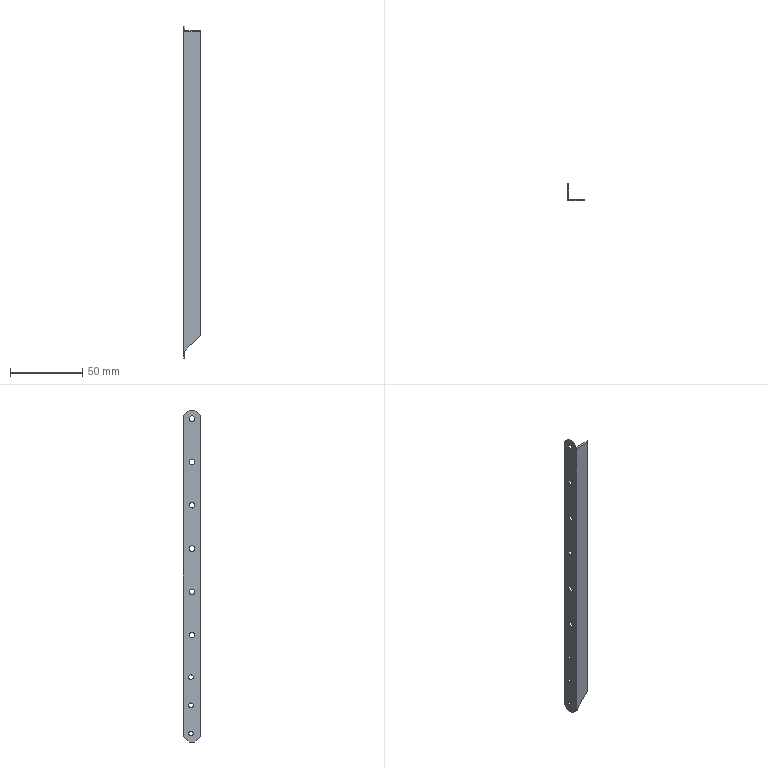Part | SolidWorks | features BaseBody 1 | 1 solid | 34 faces | box 11.5 x 12 x 230 mm | volume 3958 mm3 | cylinder 18 | plane 16 | commonest cylinder face diameters 3.855 x12 3.2 x6
STEP:
#1=CARTESIAN_POINT('',(0.,6.,-157.927));
#2=VERTEX_POINT('',#1);
#3=CARTESIAN_POINT('',(0.,6.,-154.073));
#4=VERTEX_POINT('',#3);
#5=CARTESIAN_POINT('',(0.,6.,-156.));
#6=DIRECTION('',(-1.,0.,0.));
#7=DIRECTION('',(0.,0.,-1.));
#8=AXIS2_PLACEMENT_3D('',#5,#6,#7);
#9=CIRCLE('',#8,1.927);
#10=EDGE_CURVE('',#2,#4,#9,.T.);
#11=ORIENTED_EDGE('',*,*,#10,.T.);
#12=CARTESIAN_POINT('',(0.8,6.,-154.073));
#13=VERTEX_POINT('',#12);
#14=CARTESIAN_POINT('',(0.,6.,-154.073));
#15=DIRECTION('',(1.,0.,0.));
#16=VECTOR('',#15,1000.);
#17=LINE('',#14,#16);
#18=EDGE_CURVE('',#4,#13,#17,.T.);
#19=ORIENTED_EDGE('',*,*,#18,.T.);
#20=CARTESIAN_POINT('',(0.8,6.,-157.927));
#21=VERTEX_POINT('',#20);
#22=CARTESIAN_POINT('',(0.8,6.,-156.));
#23=DIRECTION('',(1.,0.,0.));
#24=DIRECTION('',(0.,0.,-1.));
#25=AXIS2_PLACEMENT_3D('',#22,#23,#24);
#26=CIRCLE('',#25,1.927);
#27=EDGE_CURVE('',#13,#21,#26,.T.);
#28=ORIENTED_EDGE('',*,*,#27,.T.);
#29=CARTESIAN_POINT('',(0.,6.,-157.927));
#30=DIRECTION('',(1.,0.,0.));
#31=VECTOR('',#30,1000.);
#32=LINE('',#29,#31);
#33=EDGE_CURVE('',#2,#21,#32,.T.);
#34=ORIENTED_EDGE('',*,*,#33,.F.);
#35=EDGE_LOOP('',(#11,#19,#28,#34));
#36=FACE_OUTER_BOUND('',#35,.T.);
#37=CARTESIAN_POINT('',(0.,6.,-156.));
#38=DIRECTION('',(1.,0.,0.));
#39=DIRECTION('',(0.,0.,-1.));
#40=AXIS2_PLACEMENT_3D('',#37,#38,#39);
#41=CYLINDRICAL_SURFACE('',#40,1.927);
#42=ADVANCED_FACE('',(#36),#41,.F.);
#43=CARTESIAN_POINT('',(0.,6.75,-225.6));
#44=VERTEX_POINT('',#43);
#45=CARTESIAN_POINT('',(0.,6.75,-222.4));
#46=VERTEX_POINT('',#45);
#47=CARTESIAN_POINT('',(0.,6.75,-224.));
#48=DIRECTION('',(-1.,0.,0.));
#49=DIRECTION('',(0.,0.,-1.));
#50=AXIS2_PLACEMENT_3D('',#47,#48,#49);
#51=CIRCLE('',#50,1.6);
#52=EDGE_CURVE('',#44,#46,#51,.T.);
#53=ORIENTED_EDGE('',*,*,#52,.T.);
#54=CARTESIAN_POINT('',(0.8,6.75,-222.4));
#55=VERTEX_POINT('',#54);
#56=CARTESIAN_POINT('',(0.,6.75,-222.4));
#57=DIRECTION('',(1.,0.,0.));
#58=VECTOR('',#57,1000.);
#59=LINE('',#56,#58);
#60=EDGE_CURVE('',#46,#55,#59,.T.);
#61=ORIENTED_EDGE('',*,*,#60,.T.);
#62=CARTESIAN_POINT('',(0.8,6.75,-225.6));
#63=VERTEX_POINT('',#62);
#64=CARTESIAN_POINT('',(0.8,6.75,-224.));
#65=DIRECTION('',(1.,0.,0.));
#66=DIRECTION('',(0.,0.,-1.));
#67=AXIS2_PLACEMENT_3D('',#64,#65,#66);
#68=CIRCLE('',#67,1.6);
#69=EDGE_CURVE('',#55,#63,#68,.T.);
#70=ORIENTED_EDGE('',*,*,#69,.T.);
#71=CARTESIAN_POINT('',(0.,6.75,-225.6));
#72=DIRECTION('',(1.,0.,0.));
#73=VECTOR('',#72,1000.);
#74=LINE('',#71,#73);
#75=EDGE_CURVE('',#44,#63,#74,.T.);
#76=ORIENTED_EDGE('',*,*,#75,.F.);
#77=EDGE_LOOP('',(#53,#61,#70,#76));
#78=FACE_OUTER_BOUND('',#77,.T.);
#79=CARTESIAN_POINT('',(0.,6.75,-224.));
#80=DIRECTION('',(1.,0.,0.));
#81=DIRECTION('',(0.,0.,-1.));
#82=AXIS2_PLACEMENT_3D('',#79,#80,#81);
#83=CYLINDRICAL_SURFACE('',#82,1.6);
#84=ADVANCED_FACE('',(#78),#83,.F.);
#85=CARTESIAN_POINT('',(0.,6.75,-206.156));
#86=VERTEX_POINT('',#85);
#87=CARTESIAN_POINT('',(0.,6.75,-202.956));
#88=VERTEX_POINT('',#87);
#89=CARTESIAN_POINT('',(0.,6.75,-204.556));
#90=DIRECTION('',(-1.,0.,0.));
#91=DIRECTION('',(0.,0.,-1.));
#92=AXIS2_PLACEMENT_3D('',#89,#90,#91);
#93=CIRCLE('',#92,1.6);
#94=EDGE_CURVE('',#86,#88,#93,.T.);
#95=ORIENTED_EDGE('',*,*,#94,.T.);
#96=CARTESIAN_POINT('',(0.8,6.75,-202.956));
#97=VERTEX_POINT('',#96);
#98=CARTESIAN_POINT('',(0.,6.75,-202.956));
#99=DIRECTION('',(1.,0.,0.));
#100=VECTOR('',#99,1000.);
#101=LINE('',#98,#100);
#102=EDGE_CURVE('',#88,#97,#101,.T.);
#103=ORIENTED_EDGE('',*,*,#102,.T.);
#104=CARTESIAN_POINT('',(0.8,6.75,-206.156));
#105=VERTEX_POINT('',#104);
#106=CARTESIAN_POINT('',(0.8,6.75,-204.556));
#107=DIRECTION('',(1.,0.,0.));
#108=DIRECTION('',(0.,0.,-1.));
#109=AXIS2_PLACEMENT_3D('',#106,#107,#108);
#110=CIRCLE('',#109,1.6);
#111=EDGE_CURVE('',#97,#105,#110,.T.);
#112=ORIENTED_EDGE('',*,*,#111,.T.);
#113=CARTESIAN_POINT('',(0.,6.75,-206.156));
#114=DIRECTION('',(1.,0.,0.));
#115=VECTOR('',#114,1000.);
#116=LINE('',#113,#115);
#117=EDGE_CURVE('',#86,#105,#116,.T.);
#118=ORIENTED_EDGE('',*,*,#117,.F.);
#119=EDGE_LOOP('',(#95,#103,#112,#118));
#120=FACE_OUTER_BOUND('',#119,.T.);
#121=CARTESIAN_POINT('',(0.,6.75,-204.556));
#122=DIRECTION('',(1.,0.,0.));
#123=DIRECTION('',(0.,0.,-1.));
#124=AXIS2_PLACEMENT_3D('',#121,#122,#123);
#125=CYLINDRICAL_SURFACE('',#124,1.6);
#126=ADVANCED_FACE('',(#120),#125,.F.);
#127=CARTESIAN_POINT('',(0.,6.75,-186.712));
#128=VERTEX_POINT('',#127);
#129=CARTESIAN_POINT('',(0.,6.75,-183.512));
#130=VERTEX_POINT('',#129);
#131=CARTESIAN_POINT('',(0.,6.75,-185.112));
#132=DIRECTION('',(-1.,0.,0.));
#133=DIRECTION('',(0.,0.,-1.));
#134=AXIS2_PLACEMENT_3D('',#131,#132,#133);
#135=CIRCLE('',#134,1.6);
#136=EDGE_CURVE('',#128,#130,#135,.T.);
#137=ORIENTED_EDGE('',*,*,#136,.T.);
#138=CARTESIAN_POINT('',(0.8,6.75,-183.512));
#139=VERTEX_POINT('',#138);
#140=CARTESIAN_POINT('',(0.,6.75,-183.512));
#141=DIRECTION('',(1.,0.,0.));
#142=VECTOR('',#141,1000.);
#143=LINE('',#140,#142);
#144=EDGE_CURVE('',#130,#139,#143,.T.);
#145=ORIENTED_EDGE('',*,*,#144,.T.);
#146=CARTESIAN_POINT('',(0.8,6.75,-186.712));
#147=VERTEX_POINT('',#146);
#148=CARTESIAN_POINT('',(0.8,6.75,-185.112));
#149=DIRECTION('',(1.,0.,0.));
#150=DIRECTION('',(0.,0.,-1.));
#151=AXIS2_PLACEMENT_3D('',#148,#149,#150);
#152=CIRCLE('',#151,1.6);
#153=EDGE_CURVE('',#139,#147,#152,.T.);
#154=ORIENTED_EDGE('',*,*,#153,.T.);
#155=CARTESIAN_POINT('',(0.,6.75,-186.712));
#156=DIRECTION('',(1.,0.,0.));
#157=VECTOR('',#156,1000.);
#158=LINE('',#155,#157);
#159=EDGE_CURVE('',#128,#147,#158,.T.);
#160=ORIENTED_EDGE('',*,*,#159,.F.);
#161=EDGE_LOOP('',(#137,#145,#154,#160));
#162=FACE_OUTER_BOUND('',#161,.T.);
#163=CARTESIAN_POINT('',(0.,6.75,-185.112));
#164=DIRECTION('',(1.,0.,0.));
#165=DIRECTION('',(0.,0.,-1.));
#166=AXIS2_PLACEMENT_3D('',#163,#164,#165);
#167=CYLINDRICAL_SURFACE('',#166,1.6);
#168=ADVANCED_FACE('',(#162),#167,.F.);
#169=CARTESIAN_POINT('',(0.,6.,-7.927));
#170=VERTEX_POINT('',#169);
#171=CARTESIAN_POINT('',(0.,6.,-4.073));
#172=VERTEX_POINT('',#171);
#173=CARTESIAN_POINT('',(0.,6.,-6.));
#174=DIRECTION('',(-1.,0.,0.));
#175=DIRECTION('',(0.,0.,-1.));
#176=AXIS2_PLACEMENT_3D('',#173,#174,#175);
#177=CIRCLE('',#176,1.927);
#178=EDGE_CURVE('',#170,#172,#177,.T.);
#179=ORIENTED_EDGE('',*,*,#178,.T.);
#180=CARTESIAN_POINT('',(0.8,6.,-4.073));
#181=VERTEX_POINT('',#180);
#182=CARTESIAN_POINT('',(0.,6.,-4.073));
#183=DIRECTION('',(1.,0.,0.));
#184=VECTOR('',#183,1000.);
#185=LINE('',#182,#184);
#186=EDGE_CURVE('',#172,#181,#185,.T.);
#187=ORIENTED_EDGE('',*,*,#186,.T.);
#188=CARTESIAN_POINT('',(0.8,6.,-7.927));
#189=VERTEX_POINT('',#188);
#190=CARTESIAN_POINT('',(0.8,6.,-6.));
#191=DIRECTION('',(1.,0.,0.));
#192=DIRECTION('',(0.,0.,-1.));
#193=AXIS2_PLACEMENT_3D('',#190,#191,#192);
#194=CIRCLE('',#193,1.927);
#195=EDGE_CURVE('',#181,#189,#194,.T.);
#196=ORIENTED_EDGE('',*,*,#195,.T.);
#197=CARTESIAN_POINT('',(0.,6.,-7.927));
#198=DIRECTION('',(1.,0.,0.));
#199=VECTOR('',#198,1000.);
#200=LINE('',#197,#199);
#201=EDGE_CURVE('',#170,#189,#200,.T.);
#202=ORIENTED_EDGE('',*,*,#201,.F.);
#203=EDGE_LOOP('',(#179,#187,#196,#202));
#204=FACE_OUTER_BOUND('',#203,.T.);
#205=CARTESIAN_POINT('',(0.,6.,-6.));
#206=DIRECTION('',(1.,0.,0.));
#207=DIRECTION('',(0.,0.,-1.));
#208=AXIS2_PLACEMENT_3D('',#205,#206,#207);
#209=CYLINDRICAL_SURFACE('',#208,1.927);
#210=ADVANCED_FACE('',(#204),#209,.F.);
#211=CARTESIAN_POINT('',(0.,6.,-37.927));
#212=VERTEX_POINT('',#211);
#213=CARTESIAN_POINT('',(0.,6.,-34.073));
#214=VERTEX_POINT('',#213);
#215=CARTESIAN_POINT('',(0.,6.,-36.));
#216=DIRECTION('',(-1.,0.,0.));
#217=DIRECTION('',(0.,0.,-1.));
#218=AXIS2_PLACEMENT_3D('',#215,#216,#217);
#219=CIRCLE('',#218,1.927);
#220=EDGE_CURVE('',#212,#214,#219,.T.);
#221=ORIENTED_EDGE('',*,*,#220,.T.);
#222=CARTESIAN_POINT('',(0.8,6.,-34.073));
#223=VERTEX_POINT('',#222);
#224=CARTESIAN_POINT('',(0.,6.,-34.073));
#225=DIRECTION('',(1.,0.,0.));
#226=VECTOR('',#225,1000.);
#227=LINE('',#224,#226);
#228=EDGE_CURVE('',#214,#223,#227,.T.);
#229=ORIENTED_EDGE('',*,*,#228,.T.);
#230=CARTESIAN_POINT('',(0.8,6.,-37.927));
#231=VERTEX_POINT('',#230);
#232=CARTESIAN_POINT('',(0.8,6.,-36.));
#233=DIRECTION('',(1.,0.,0.));
#234=DIRECTION('',(0.,0.,-1.));
#235=AXIS2_PLACEMENT_3D('',#232,#233,#234);
#236=CIRCLE('',#235,1.927);
#237=EDGE_CURVE('',#223,#231,#236,.T.);
#238=ORIENTED_EDGE('',*,*,#237,.T.);
#239=CARTESIAN_POINT('',(0.,6.,-37.927));
#240=DIRECTION('',(1.,0.,0.));
#241=VECTOR('',#240,1000.);
#242=LINE('',#239,#241);
#243=EDGE_CURVE('',#212,#231,#242,.T.);
#244=ORIENTED_EDGE('',*,*,#243,.F.);
#245=EDGE_LOOP('',(#221,#229,#238,#244));
#246=FACE_OUTER_BOUND('',#245,.T.);
#247=CARTESIAN_POINT('',(0.,6.,-36.));
#248=DIRECTION('',(1.,0.,0.));
#249=DIRECTION('',(0.,0.,-1.));
#250=AXIS2_PLACEMENT_3D('',#247,#248,#249);
#251=CYLINDRICAL_SURFACE('',#250,1.927);
#252=ADVANCED_FACE('',(#246),#251,.F.);
#253=CARTESIAN_POINT('',(0.,6.,-67.927));
#254=VERTEX_POINT('',#253);
#255=CARTESIAN_POINT('',(0.,6.,-64.073));
#256=VERTEX_POINT('',#255);
#257=CARTESIAN_POINT('',(0.,6.,-66.));
#258=DIRECTION('',(-1.,0.,0.));
#259=DIRECTION('',(0.,0.,-1.));
#260=AXIS2_PLACEMENT_3D('',#257,#258,#259);
#261=CIRCLE('',#260,1.927);
#262=EDGE_CURVE('',#254,#256,#261,.T.);
#263=ORIENTED_EDGE('',*,*,#262,.T.);
#264=CARTESIAN_POINT('',(0.8,6.,-64.073));
#265=VERTEX_POINT('',#264);
#266=CARTESIAN_POINT('',(0.,6.,-64.073));
#267=DIRECTION('',(1.,0.,0.));
#268=VECTOR('',#267,1000.);
#269=LINE('',#266,#268);
#270=EDGE_CURVE('',#256,#265,#269,.T.);
#271=ORIENTED_EDGE('',*,*,#270,.T.);
#272=CARTESIAN_POINT('',(0.8,6.,-67.927));
#273=VERTEX_POINT('',#272);
#274=CARTESIAN_POINT('',(0.8,6.,-66.));
#275=DIRECTION('',(1.,0.,0.));
#276=DIRECTION('',(0.,0.,-1.));
#277=AXIS2_PLACEMENT_3D('',#274,#275,#276);
#278=CIRCLE('',#277,1.927);
#279=EDGE_CURVE('',#265,#273,#278,.T.);
#280=ORIENTED_EDGE('',*,*,#279,.T.);
#281=CARTESIAN_POINT('',(0.,6.,-67.927));
#282=DIRECTION('',(1.,0.,0.));
#283=VECTOR('',#282,1000.);
#284=LINE('',#281,#283);
#285=EDGE_CURVE('',#254,#273,#284,.T.);
#286=ORIENTED_EDGE('',*,*,#285,.F.);
#287=EDGE_LOOP('',(#263,#271,#280,#286));
#288=FACE_OUTER_BOUND('',#287,.T.);
#289=CARTESIAN_POINT('',(0.,6.,-66.));
#290=DIRECTION('',(1.,0.,0.));
#291=DIRECTION('',(0.,0.,-1.));
#292=AXIS2_PLACEMENT_3D('',#289,#290,#291);
#293=CYLINDRICAL_SURFACE('',#292,1.927);
#294=ADVANCED_FACE('',(#288),#293,.F.);
#295=CARTESIAN_POINT('',(0.,6.,-97.927));
#296=VERTEX_POINT('',#295);
#297=CARTESIAN_POINT('',(0.,6.,-94.073));
#298=VERTEX_POINT('',#297);
#299=CARTESIAN_POINT('',(0.,6.,-96.));
#300=DIRECTION('',(-1.,0.,0.));
#301=DIRECTION('',(0.,0.,-1.));
#302=AXIS2_PLACEMENT_3D('',#299,#300,#301);
#303=CIRCLE('',#302,1.927);
#304=EDGE_CURVE('',#296,#298,#303,.T.);
#305=ORIENTED_EDGE('',*,*,#304,.T.);
#306=CARTESIAN_POINT('',(0.8,6.,-94.073));
#307=VERTEX_POINT('',#306);
#308=CARTESIAN_POINT('',(0.,6.,-94.073));
#309=DIRECTION('',(1.,0.,0.));
#310=VECTOR('',#309,1000.);
#311=LINE('',#308,#310);
#312=EDGE_CURVE('',#298,#307,#311,.T.);
#313=ORIENTED_EDGE('',*,*,#312,.T.);
#314=CARTESIAN_POINT('',(0.8,6.,-97.927));
#315=VERTEX_POINT('',#314);
#316=CARTESIAN_POINT('',(0.8,6.,-96.));
#317=DIRECTION('',(1.,0.,0.));
#318=DIRECTION('',(0.,0.,-1.));
#319=AXIS2_PLACEMENT_3D('',#316,#317,#318);
#320=CIRCLE('',#319,1.927);
#321=EDGE_CURVE('',#307,#315,#320,.T.);
#322=ORIENTED_EDGE('',*,*,#321,.T.);
#323=CARTESIAN_POINT('',(0.,6.,-97.927));
#324=DIRECTION('',(1.,0.,0.));
#325=VECTOR('',#324,1000.);
#326=LINE('',#323,#325);
#327=EDGE_CURVE('',#296,#315,#326,.T.);
#328=ORIENTED_EDGE('',*,*,#327,.F.);
#329=EDGE_LOOP('',(#305,#313,#322,#328));
#330=FACE_OUTER_BOUND('',#329,.T.);
#331=CARTESIAN_POINT('',(0.,6.,-96.));
#332=DIRECTION('',(1.,0.,0.));
#333=DIRECTION('',(0.,0.,-1.));
#334=AXIS2_PLACEMENT_3D('',#331,#332,#333);
#335=CYLINDRICAL_SURFACE('',#334,1.927);
#336=ADVANCED_FACE('',(#330),#335,.F.);
#337=CARTESIAN_POINT('',(0.,6.,-127.927));
#338=VERTEX_POINT('',#337);
#339=CARTESIAN_POINT('',(0.,6.,-124.073));
#340=VERTEX_POINT('',#339);
#341=CARTESIAN_POINT('',(0.,6.,-126.));
#342=DIRECTION('',(-1.,0.,0.));
#343=DIRECTION('',(0.,0.,-1.));
#344=AXIS2_PLACEMENT_3D('',#341,#342,#343);
#345=CIRCLE('',#344,1.927);
#346=EDGE_CURVE('',#338,#340,#345,.T.);
#347=ORIENTED_EDGE('',*,*,#346,.T.);
#348=CARTESIAN_POINT('',(0.8,6.,-124.073));
#349=VERTEX_POINT('',#348);
#350=CARTESIAN_POINT('',(0.,6.,-124.073));
#351=DIRECTION('',(1.,0.,0.));
#352=VECTOR('',#351,1000.);
#353=LINE('',#350,#352);
#354=EDGE_CURVE('',#340,#349,#353,.T.);
#355=ORIENTED_EDGE('',*,*,#354,.T.);
#356=CARTESIAN_POINT('',(0.8,6.,-127.927));
#357=VERTEX_POINT('',#356);
#358=CARTESIAN_POINT('',(0.8,6.,-126.));
#359=DIRECTION('',(1.,0.,0.));
#360=DIRECTION('',(0.,0.,-1.));
#361=AXIS2_PLACEMENT_3D('',#358,#359,#360);
#362=CIRCLE('',#361,1.927);
#363=EDGE_CURVE('',#349,#357,#362,.T.);
#364=ORIENTED_EDGE('',*,*,#363,.T.);
#365=CARTESIAN_POINT('',(0.,6.,-127.927));
#366=DIRECTION('',(1.,0.,0.));
#367=VECTOR('',#366,1000.);
#368=LINE('',#365,#367);
#369=EDGE_CURVE('',#338,#357,#368,.T.);
#370=ORIENTED_EDGE('',*,*,#369,.F.);
#371=EDGE_LOOP('',(#347,#355,#364,#370));
#372=FACE_OUTER_BOUND('',#371,.T.);
#373=CARTESIAN_POINT('',(0.,6.,-126.));
#374=DIRECTION('',(1.,0.,0.));
#375=DIRECTION('',(0.,0.,-1.));
#376=AXIS2_PLACEMENT_3D('',#373,#374,#375);
#377=CYLINDRICAL_SURFACE('',#376,1.927);
#378=ADVANCED_FACE('',(#372),#377,.F.);
#379=ORIENTED_EDGE('',*,*,#18,.F.);
#380=CARTESIAN_POINT('',(0.,6.,-156.));
#381=DIRECTION('',(-1.,0.,0.));
#382=DIRECTION('',(0.,0.,-1.));
#383=AXIS2_PLACEMENT_3D('',#380,#381,#382);
#384=CIRCLE('',#383,1.927);
#385=EDGE_CURVE('',#4,#2,#384,.T.);
#386=ORIENTED_EDGE('',*,*,#385,.T.);
#387=ORIENTED_EDGE('',*,*,#33,.T.);
#388=CARTESIAN_POINT('',(0.8,6.,-156.));
#389=DIRECTION('',(1.,0.,0.));
#390=DIRECTION('',(0.,0.,-1.));
#391=AXIS2_PLACEMENT_3D('',#388,#389,#390);
#392=CIRCLE('',#391,1.927);
#393=EDGE_CURVE('',#21,#13,#392,.T.);
#394=ORIENTED_EDGE('',*,*,#393,.T.);
#395=EDGE_LOOP('',(#379,#386,#387,#394));
#396=FACE_OUTER_BOUND('',#395,.T.);
#397=CARTESIAN_POINT('',(0.,6.,-156.));
#398=DIRECTION('',(1.,0.,0.));
#399=DIRECTION('',(0.,0.,-1.));
#400=AXIS2_PLACEMENT_3D('',#397,#398,#399);
#401=CYLINDRICAL_SURFACE('',#400,1.927);
#402=ADVANCED_FACE('',(#396),#401,.F.);
#403=CARTESIAN_POINT('',(0.8,6.75,-224.));
#404=DIRECTION('',(1.,0.,0.));
#405=DIRECTION('',(0.,0.,-1.));
#406=AXIS2_PLACEMENT_3D('',#403,#404,#405);
#407=CIRCLE('',#406,1.6);
#408=EDGE_CURVE('',#63,#55,#407,.T.);
#409=ORIENTED_EDGE('',*,*,#408,.F.);
#410=ORIENTED_EDGE('',*,*,#69,.F.);
#411=EDGE_LOOP('',(#409,#410));
#412=FACE_BOUND('',#411,.T.);
#413=CARTESIAN_POINT('',(0.8,6.75,-204.556));
#414=DIRECTION('',(1.,0.,0.));
#415=DIRECTION('',(0.,0.,-1.));
#416=AXIS2_PLACEMENT_3D('',#413,#414,#415);
#417=CIRCLE('',#416,1.6);
#418=EDGE_CURVE('',#105,#97,#417,.T.);
#419=ORIENTED_EDGE('',*,*,#418,.F.);
#420=ORIENTED_EDGE('',*,*,#111,.F.);
#421=EDGE_LOOP('',(#419,#420));
#422=FACE_BOUND('',#421,.T.);
#423=CARTESIAN_POINT('',(0.8,6.75,-185.112));
#424=DIRECTION('',(1.,0.,0.));
#425=DIRECTION('',(0.,0.,-1.));
#426=AXIS2_PLACEMENT_3D('',#423,#424,#425);
#427=CIRCLE('',#426,1.6);
#428=EDGE_CURVE('',#147,#139,#427,.T.);
#429=ORIENTED_EDGE('',*,*,#428,.F.);
#430=ORIENTED_EDGE('',*,*,#153,.F.);
#431=EDGE_LOOP('',(#429,#430));
#432=FACE_BOUND('',#431,.T.);
#433=CARTESIAN_POINT('',(0.8,6.,-6.));
#434=DIRECTION('',(1.,0.,0.));
#435=DIRECTION('',(0.,0.,-1.));
#436=AXIS2_PLACEMENT_3D('',#433,#434,#435);
#437=CIRCLE('',#436,1.927);
#438=EDGE_CURVE('',#189,#181,#437,.T.);
#439=ORIENTED_EDGE('',*,*,#438,.F.);
#440=ORIENTED_EDGE('',*,*,#195,.F.);
#441=EDGE_LOOP('',(#439,#440));
#442=FACE_BOUND('',#441,.T.);
#443=CARTESIAN_POINT('',(0.8,6.,-36.));
#444=DIRECTION('',(1.,0.,0.));
#445=DIRECTION('',(0.,0.,-1.));
#446=AXIS2_PLACEMENT_3D('',#443,#444,#445);
#447=CIRCLE('',#446,1.927);
#448=EDGE_CURVE('',#231,#223,#447,.T.);
#449=ORIENTED_EDGE('',*,*,#448,.F.);
#450=ORIENTED_EDGE('',*,*,#237,.F.);
#451=EDGE_LOOP('',(#449,#450));
#452=FACE_BOUND('',#451,.T.);
#453=CARTESIAN_POINT('',(0.8,6.,-66.));
#454=DIRECTION('',(1.,0.,0.));
#455=DIRECTION('',(0.,0.,-1.));
#456=AXIS2_PLACEMENT_3D('',#453,#454,#455);
#457=CIRCLE('',#456,1.927);
#458=EDGE_CURVE('',#273,#265,#457,.T.);
#459=ORIENTED_EDGE('',*,*,#458,.F.);
#460=ORIENTED_EDGE('',*,*,#279,.F.);
#461=EDGE_LOOP('',(#459,#460));
#462=FACE_BOUND('',#461,.T.);
#463=CARTESIAN_POINT('',(0.8,6.,-96.));
#464=DIRECTION('',(1.,0.,0.));
#465=DIRECTION('',(0.,0.,-1.));
#466=AXIS2_PLACEMENT_3D('',#463,#464,#465);
#467=CIRCLE('',#466,1.927);
#468=EDGE_CURVE('',#315,#307,#467,.T.);
#469=ORIENTED_EDGE('',*,*,#468,.F.);
#470=ORIENTED_EDGE('',*,*,#321,.F.);
#471=EDGE_LOOP('',(#469,#470));
#472=FACE_BOUND('',#471,.T.);
#473=CARTESIAN_POINT('',(0.8,6.,-126.));
#474=DIRECTION('',(1.,0.,0.));
#475=DIRECTION('',(0.,0.,-1.));
#476=AXIS2_PLACEMENT_3D('',#473,#474,#475);
#477=CIRCLE('',#476,1.927);
#478=EDGE_CURVE('',#357,#349,#477,.T.);
#479=ORIENTED_EDGE('',*,*,#478,.F.);
#480=ORIENTED_EDGE('',*,*,#363,.F.);
#481=EDGE_LOOP('',(#479,#480));
#482=FACE_BOUND('',#481,.T.);
#483=ORIENTED_EDGE('',*,*,#393,.F.);
#484=ORIENTED_EDGE('',*,*,#27,.F.);
#485=EDGE_LOOP('',(#483,#484));
#486=FACE_BOUND('',#485,.T.);
#487=CARTESIAN_POINT('',(0.8,8.,0.));
#488=VERTEX_POINT('',#487);
#489=CARTESIAN_POINT('',(0.8,12.,-4.));
#490=VERTEX_POINT('',#489);
#491=CARTESIAN_POINT('',(0.8,8.,0.));
#492=DIRECTION('',(0.,0.7071,-0.7071));
#493=VECTOR('',#492,1000.);
#494=LINE('',#491,#493);
#495=EDGE_CURVE('',#488,#490,#494,.T.);
#496=ORIENTED_EDGE('',*,*,#495,.F.);
#497=CARTESIAN_POINT('',(0.8,4.,0.));
#498=VERTEX_POINT('',#497);
#499=CARTESIAN_POINT('',(0.8,6.4,0.));
#500=DIRECTION('',(0.,1.,0.));
#501=VECTOR('',#500,1000.);
#502=LINE('',#499,#501);
#503=EDGE_CURVE('',#498,#488,#502,.T.);
#504=ORIENTED_EDGE('',*,*,#503,.F.);
#505=CARTESIAN_POINT('',(0.8,0.8,-3.2));
#506=VERTEX_POINT('',#505);
#507=CARTESIAN_POINT('',(0.8,0.,-4.));
#508=DIRECTION('',(0.,0.7071,0.7071));
#509=VECTOR('',#508,1000.);
#510=LINE('',#507,#509);
#511=EDGE_CURVE('',#506,#498,#510,.T.);
#512=ORIENTED_EDGE('',*,*,#511,.F.);
#513=CARTESIAN_POINT('',(0.8,0.8,-225.165));
#514=VERTEX_POINT('',#513);
#515=CARTESIAN_POINT('',(0.8,0.8,-115.));
#516=DIRECTION('',(0.,0.,1.));
#517=VECTOR('',#516,1000.);
#518=LINE('',#515,#517);
#519=EDGE_CURVE('',#514,#506,#518,.T.);
#520=ORIENTED_EDGE('',*,*,#519,.F.);
#521=CARTESIAN_POINT('',(0.8,0.8,-226.8));
#522=VERTEX_POINT('',#521);
#523=CARTESIAN_POINT('',(0.8,0.8,-115.));
#524=DIRECTION('',(0.,0.,1.));
#525=VECTOR('',#524,1000.);
#526=LINE('',#523,#525);
#527=EDGE_CURVE('',#522,#514,#526,.T.);
#528=ORIENTED_EDGE('',*,*,#527,.F.);
#529=CARTESIAN_POINT('',(0.8,4.,-230.));
#530=VERTEX_POINT('',#529);
#531=CARTESIAN_POINT('',(0.8,0.,-226.));
#532=DIRECTION('',(0.,-0.7071,0.7071));
#533=VECTOR('',#532,1000.);
#534=LINE('',#531,#533);
#535=EDGE_CURVE('',#530,#522,#534,.T.);
#536=ORIENTED_EDGE('',*,*,#535,.F.);
#537=CARTESIAN_POINT('',(0.8,8.,-230.));
#538=VERTEX_POINT('',#537);
#539=CARTESIAN_POINT('',(0.8,6.4,-230.));
#540=DIRECTION('',(0.,-1.,0.));
#541=VECTOR('',#540,1000.);
#542=LINE('',#539,#541);
#543=EDGE_CURVE('',#538,#530,#542,.T.);
#544=ORIENTED_EDGE('',*,*,#543,.F.);
#545=CARTESIAN_POINT('',(0.8,12.,-226.));
#546=VERTEX_POINT('',#545);
#547=CARTESIAN_POINT('',(0.8,8.,-230.));
#548=DIRECTION('',(0.,-0.7071,-0.7071));
#549=VECTOR('',#548,1000.);
#550=LINE('',#547,#549);
#551=EDGE_CURVE('',#546,#538,#550,.T.);
#552=ORIENTED_EDGE('',*,*,#551,.F.);
#553=CARTESIAN_POINT('',(0.8,12.,-115.));
#554=DIRECTION('',(0.,0.,-1.));
#555=VECTOR('',#554,1000.);
#556=LINE('',#553,#555);
#557=EDGE_CURVE('',#490,#546,#556,.T.);
#558=ORIENTED_EDGE('',*,*,#557,.F.);
#559=EDGE_LOOP('',(#496,#504,#512,#520,#528,#536,#544,#552,#558));
#560=FACE_OUTER_BOUND('',#559,.T.);
#561=CARTESIAN_POINT('',(0.8,12.,0.));
#562=DIRECTION('',(-1.,0.,0.));
#563=DIRECTION('',(0.,0.,-1.));
#564=AXIS2_PLACEMENT_3D('',#561,#562,#563);
#565=PLANE('',#564);
#566=ADVANCED_FACE('',(#412,#422,#432,#442,#452,#462,#472,#482,#486,#560),#565,.F.);
#567=ORIENTED_EDGE('',*,*,#52,.F.);
#568=CARTESIAN_POINT('',(0.,6.75,-224.));
#569=DIRECTION('',(-1.,0.,0.));
#570=DIRECTION('',(0.,0.,-1.));
#571=AXIS2_PLACEMENT_3D('',#568,#569,#570);
#572=CIRCLE('',#571,1.6);
#573=EDGE_CURVE('',#46,#44,#572,.T.);
#574=ORIENTED_EDGE('',*,*,#573,.F.);
#575=EDGE_LOOP('',(#567,#574));
#576=FACE_BOUND('',#575,.T.);
#577=ORIENTED_EDGE('',*,*,#94,.F.);
#578=CARTESIAN_POINT('',(0.,6.75,-204.556));
#579=DIRECTION('',(-1.,0.,0.));
#580=DIRECTION('',(0.,0.,-1.));
#581=AXIS2_PLACEMENT_3D('',#578,#579,#580);
#582=CIRCLE('',#581,1.6);
#583=EDGE_CURVE('',#88,#86,#582,.T.);
#584=ORIENTED_EDGE('',*,*,#583,.F.);
#585=EDGE_LOOP('',(#577,#584));
#586=FACE_BOUND('',#585,.T.);
#587=ORIENTED_EDGE('',*,*,#136,.F.);
#588=CARTESIAN_POINT('',(0.,6.75,-185.112));
#589=DIRECTION('',(-1.,0.,0.));
#590=DIRECTION('',(0.,0.,-1.));
#591=AXIS2_PLACEMENT_3D('',#588,#589,#590);
#592=CIRCLE('',#591,1.6);
#593=EDGE_CURVE('',#130,#128,#592,.T.);
#594=ORIENTED_EDGE('',*,*,#593,.F.);
#595=EDGE_LOOP('',(#587,#594));
#596=FACE_BOUND('',#595,.T.);
#597=ORIENTED_EDGE('',*,*,#178,.F.);
#598=CARTESIAN_POINT('',(0.,6.,-6.));
#599=DIRECTION('',(-1.,0.,0.));
#600=DIRECTION('',(0.,0.,-1.));
#601=AXIS2_PLACEMENT_3D('',#598,#599,#600);
#602=CIRCLE('',#601,1.927);
#603=EDGE_CURVE('',#172,#170,#602,.T.);
#604=ORIENTED_EDGE('',*,*,#603,.F.);
#605=EDGE_LOOP('',(#597,#604));
#606=FACE_BOUND('',#605,.T.);
#607=ORIENTED_EDGE('',*,*,#220,.F.);
#608=CARTESIAN_POINT('',(0.,6.,-36.));
#609=DIRECTION('',(-1.,0.,0.));
#610=DIRECTION('',(0.,0.,-1.));
#611=AXIS2_PLACEMENT_3D('',#608,#609,#610);
#612=CIRCLE('',#611,1.927);
#613=EDGE_CURVE('',#214,#212,#612,.T.);
#614=ORIENTED_EDGE('',*,*,#613,.F.);
#615=EDGE_LOOP('',(#607,#614));
#616=FACE_BOUND('',#615,.T.);
#617=ORIENTED_EDGE('',*,*,#262,.F.);
#618=CARTESIAN_POINT('',(0.,6.,-66.));
#619=DIRECTION('',(-1.,0.,0.));
#620=DIRECTION('',(0.,0.,-1.));
#621=AXIS2_PLACEMENT_3D('',#618,#619,#620);
#622=CIRCLE('',#621,1.927);
#623=EDGE_CURVE('',#256,#254,#622,.T.);
#624=ORIENTED_EDGE('',*,*,#623,.F.);
#625=EDGE_LOOP('',(#617,#624));
#626=FACE_BOUND('',#625,.T.);
#627=ORIENTED_EDGE('',*,*,#304,.F.);
#628=CARTESIAN_POINT('',(0.,6.,-96.));
#629=DIRECTION('',(-1.,0.,0.));
#630=DIRECTION('',(0.,0.,-1.));
#631=AXIS2_PLACEMENT_3D('',#628,#629,#630);
#632=CIRCLE('',#631,1.927);
#633=EDGE_CURVE('',#298,#296,#632,.T.);
#634=ORIENTED_EDGE('',*,*,#633,.F.);
#635=EDGE_LOOP('',(#627,#634));
#636=FACE_BOUND('',#635,.T.);
#637=ORIENTED_EDGE('',*,*,#346,.F.);
#638=CARTESIAN_POINT('',(0.,6.,-126.));
#639=DIRECTION('',(-1.,0.,0.));
#640=DIRECTION('',(0.,0.,-1.));
#641=AXIS2_PLACEMENT_3D('',#638,#639,#640);
#642=CIRCLE('',#641,1.927);
#643=EDGE_CURVE('',#340,#338,#642,.T.);
#644=ORIENTED_EDGE('',*,*,#643,.F.);
#645=EDGE_LOOP('',(#637,#644));
#646=FACE_BOUND('',#645,.T.);
#647=ORIENTED_EDGE('',*,*,#10,.F.);
#648=ORIENTED_EDGE('',*,*,#385,.F.);
#649=EDGE_LOOP('',(#647,#648));
#650=FACE_BOUND('',#649,.T.);
#651=CARTESIAN_POINT('',(0.,0.,-226.));
#652=VERTEX_POINT('',#651);
#653=CARTESIAN_POINT('',(0.,4.,-230.));
#654=VERTEX_POINT('',#653);
#655=CARTESIAN_POINT('',(0.,0.,-226.));
#656=DIRECTION('',(0.,0.7071,-0.7071));
#657=VECTOR('',#656,1000.);
#658=LINE('',#655,#657);
#659=EDGE_CURVE('',#652,#654,#658,.T.);
#660=ORIENTED_EDGE('',*,*,#659,.F.);
#661=CARTESIAN_POINT('',(0.,0.,-4.));
#662=VERTEX_POINT('',#661);
#663=CARTESIAN_POINT('',(0.,0.,-115.));
#664=DIRECTION('',(0.,0.,-1.));
#665=VECTOR('',#664,1000.);
#666=LINE('',#663,#665);
#667=EDGE_CURVE('',#662,#652,#666,.T.);
#668=ORIENTED_EDGE('',*,*,#667,.F.);
#669=CARTESIAN_POINT('',(0.,4.,0.));
#670=VERTEX_POINT('',#669);
#671=CARTESIAN_POINT('',(0.,0.,-4.));
#672=DIRECTION('',(0.,-0.7071,-0.7071));
#673=VECTOR('',#672,1000.);
#674=LINE('',#671,#673);
#675=EDGE_CURVE('',#670,#662,#674,.T.);
#676=ORIENTED_EDGE('',*,*,#675,.F.);
#677=CARTESIAN_POINT('',(0.,8.,0.));
#678=VERTEX_POINT('',#677);
#679=CARTESIAN_POINT('',(0.,6.,0.));
#680=DIRECTION('',(0.,-1.,0.));
#681=VECTOR('',#680,1000.);
#682=LINE('',#679,#681);
#683=EDGE_CURVE('',#678,#670,#682,.T.);
#684=ORIENTED_EDGE('',*,*,#683,.F.);
#685=CARTESIAN_POINT('',(0.,12.,-4.));
#686=VERTEX_POINT('',#685);
#687=CARTESIAN_POINT('',(0.,8.,0.));
#688=DIRECTION('',(0.,-0.7071,0.7071));
#689=VECTOR('',#688,1000.);
#690=LINE('',#687,#689);
#691=EDGE_CURVE('',#686,#678,#690,.T.);
#692=ORIENTED_EDGE('',*,*,#691,.F.);
#693=CARTESIAN_POINT('',(0.,12.,-226.));
#694=VERTEX_POINT('',#693);
#695=CARTESIAN_POINT('',(0.,12.,-115.));
#696=DIRECTION('',(0.,0.,1.));
#697=VECTOR('',#696,1000.);
#698=LINE('',#695,#697);
#699=EDGE_CURVE('',#694,#686,#698,.T.);
#700=ORIENTED_EDGE('',*,*,#699,.F.);
#701=CARTESIAN_POINT('',(0.,8.,-230.));
#702=VERTEX_POINT('',#701);
#703=CARTESIAN_POINT('',(0.,8.,-230.));
#704=DIRECTION('',(0.,0.7071,0.7071));
#705=VECTOR('',#704,1000.);
#706=LINE('',#703,#705);
#707=EDGE_CURVE('',#702,#694,#706,.T.);
#708=ORIENTED_EDGE('',*,*,#707,.F.);
#709=CARTESIAN_POINT('',(0.,6.,-230.));
#710=DIRECTION('',(0.,1.,0.));
#711=VECTOR('',#710,1000.);
#712=LINE('',#709,#711);
#713=EDGE_CURVE('',#654,#702,#712,.T.);
#714=ORIENTED_EDGE('',*,*,#713,.F.);
#715=EDGE_LOOP('',(#660,#668,#676,#684,#692,#700,#708,#714));
#716=FACE_OUTER_BOUND('',#715,.T.);
#717=CARTESIAN_POINT('',(0.,0.,-230.));
#718=DIRECTION('',(1.,0.,0.));
#719=DIRECTION('',(0.,1.,0.));
#720=AXIS2_PLACEMENT_3D('',#717,#718,#719);
#721=PLANE('',#720);
#722=ADVANCED_FACE('',(#576,#586,#596,#606,#616,#626,#636,#646,#650,#716),#721,.F.);
#723=ORIENTED_EDGE('',*,*,#60,.F.);
#724=ORIENTED_EDGE('',*,*,#573,.T.);
#725=ORIENTED_EDGE('',*,*,#75,.T.);
#726=ORIENTED_EDGE('',*,*,#408,.T.);
#727=EDGE_LOOP('',(#723,#724,#725,#726));
#728=FACE_OUTER_BOUND('',#727,.T.);
#729=CARTESIAN_POINT('',(0.,6.75,-224.));
#730=DIRECTION('',(1.,0.,0.));
#731=DIRECTION('',(0.,0.,-1.));
#732=AXIS2_PLACEMENT_3D('',#729,#730,#731);
#733=CYLINDRICAL_SURFACE('',#732,1.6);
#734=ADVANCED_FACE('',(#728),#733,.F.);
#735=ORIENTED_EDGE('',*,*,#102,.F.);
#736=ORIENTED_EDGE('',*,*,#583,.T.);
#737=ORIENTED_EDGE('',*,*,#117,.T.);
#738=ORIENTED_EDGE('',*,*,#418,.T.);
#739=EDGE_LOOP('',(#735,#736,#737,#738));
#740=FACE_OUTER_BOUND('',#739,.T.);
#741=CARTESIAN_POINT('',(0.,6.75,-204.556));
#742=DIRECTION('',(1.,0.,0.));
#743=DIRECTION('',(0.,0.,-1.));
#744=AXIS2_PLACEMENT_3D('',#741,#742,#743);
#745=CYLINDRICAL_SURFACE('',#744,1.6);
#746=ADVANCED_FACE('',(#740),#745,.F.);
#747=ORIENTED_EDGE('',*,*,#144,.F.);
#748=ORIENTED_EDGE('',*,*,#593,.T.);
#749=ORIENTED_EDGE('',*,*,#159,.T.);
#750=ORIENTED_EDGE('',*,*,#428,.T.);
#751=EDGE_LOOP('',(#747,#748,#749,#750));
#752=FACE_OUTER_BOUND('',#751,.T.);
#753=CARTESIAN_POINT('',(0.,6.75,-185.112));
#754=DIRECTION('',(1.,0.,0.));
#755=DIRECTION('',(0.,0.,-1.));
#756=AXIS2_PLACEMENT_3D('',#753,#754,#755);
#757=CYLINDRICAL_SURFACE('',#756,1.6);
#758=ADVANCED_FACE('',(#752),#757,.F.);
#759=ORIENTED_EDGE('',*,*,#186,.F.);
#760=ORIENTED_EDGE('',*,*,#603,.T.);
#761=ORIENTED_EDGE('',*,*,#201,.T.);
#762=ORIENTED_EDGE('',*,*,#438,.T.);
#763=EDGE_LOOP('',(#759,#760,#761,#762));
#764=FACE_OUTER_BOUND('',#763,.T.);
#765=CARTESIAN_POINT('',(0.,6.,-6.));
#766=DIRECTION('',(1.,0.,0.));
#767=DIRECTION('',(0.,0.,-1.));
#768=AXIS2_PLACEMENT_3D('',#765,#766,#767);
#769=CYLINDRICAL_SURFACE('',#768,1.927);
#770=ADVANCED_FACE('',(#764),#769,.F.);
#771=ORIENTED_EDGE('',*,*,#228,.F.);
#772=ORIENTED_EDGE('',*,*,#613,.T.);
#773=ORIENTED_EDGE('',*,*,#243,.T.);
#774=ORIENTED_EDGE('',*,*,#448,.T.);
#775=EDGE_LOOP('',(#771,#772,#773,#774));
#776=FACE_OUTER_BOUND('',#775,.T.);
#777=CARTESIAN_POINT('',(0.,6.,-36.));
#778=DIRECTION('',(1.,0.,0.));
#779=DIRECTION('',(0.,0.,-1.));
#780=AXIS2_PLACEMENT_3D('',#777,#778,#779);
#781=CYLINDRICAL_SURFACE('',#780,1.927);
#782=ADVANCED_FACE('',(#776),#781,.F.);
#783=ORIENTED_EDGE('',*,*,#270,.F.);
#784=ORIENTED_EDGE('',*,*,#623,.T.);
#785=ORIENTED_EDGE('',*,*,#285,.T.);
#786=ORIENTED_EDGE('',*,*,#458,.T.);
#787=EDGE_LOOP('',(#783,#784,#785,#786));
#788=FACE_OUTER_BOUND('',#787,.T.);
#789=CARTESIAN_POINT('',(0.,6.,-66.));
#790=DIRECTION('',(1.,0.,0.));
#791=DIRECTION('',(0.,0.,-1.));
#792=AXIS2_PLACEMENT_3D('',#789,#790,#791);
#793=CYLINDRICAL_SURFACE('',#792,1.927);
#794=ADVANCED_FACE('',(#788),#793,.F.);
#795=ORIENTED_EDGE('',*,*,#312,.F.);
#796=ORIENTED_EDGE('',*,*,#633,.T.);
#797=ORIENTED_EDGE('',*,*,#327,.T.);
#798=ORIENTED_EDGE('',*,*,#468,.T.);
#799=EDGE_LOOP('',(#795,#796,#797,#798));
#800=FACE_OUTER_BOUND('',#799,.T.);
#801=CARTESIAN_POINT('',(0.,6.,-96.));
#802=DIRECTION('',(1.,0.,0.));
#803=DIRECTION('',(0.,0.,-1.));
#804=AXIS2_PLACEMENT_3D('',#801,#802,#803);
#805=CYLINDRICAL_SURFACE('',#804,1.927);
#806=ADVANCED_FACE('',(#800),#805,.F.);
#807=ORIENTED_EDGE('',*,*,#354,.F.);
#808=ORIENTED_EDGE('',*,*,#643,.T.);
#809=ORIENTED_EDGE('',*,*,#369,.T.);
#810=ORIENTED_EDGE('',*,*,#478,.T.);
#811=EDGE_LOOP('',(#807,#808,#809,#810));
#812=FACE_OUTER_BOUND('',#811,.T.);
#813=CARTESIAN_POINT('',(0.,6.,-126.));
#814=DIRECTION('',(1.,0.,0.));
#815=DIRECTION('',(0.,0.,-1.));
#816=AXIS2_PLACEMENT_3D('',#813,#814,#815);
#817=CYLINDRICAL_SURFACE('',#816,1.927);
#818=ADVANCED_FACE('',(#812),#817,.F.);
#819=CARTESIAN_POINT('',(0.4,12.,-4.));
#820=DIRECTION('',(-1.,0.,0.));
#821=VECTOR('',#820,1000.);
#822=LINE('',#819,#821);
#823=EDGE_CURVE('',#490,#686,#822,.T.);
#824=ORIENTED_EDGE('',*,*,#823,.F.);
#825=ORIENTED_EDGE('',*,*,#557,.T.);
#826=CARTESIAN_POINT('',(0.4,12.,-226.));
#827=DIRECTION('',(1.,0.,0.));
#828=VECTOR('',#827,1000.);
#829=LINE('',#826,#828);
#830=EDGE_CURVE('',#694,#546,#829,.T.);
#831=ORIENTED_EDGE('',*,*,#830,.F.);
#832=ORIENTED_EDGE('',*,*,#699,.T.);
#833=EDGE_LOOP('',(#824,#825,#831,#832));
#834=FACE_OUTER_BOUND('',#833,.T.);
#835=CARTESIAN_POINT('',(0.8,12.,-226.));
#836=DIRECTION('',(0.,-1.,0.));
#837=DIRECTION('',(0.,0.,1.));
#838=AXIS2_PLACEMENT_3D('',#835,#836,#837);
#839=PLANE('',#838);
#840=ADVANCED_FACE('',(#834),#839,.F.);
#841=ORIENTED_EDGE('',*,*,#691,.T.);
#842=CARTESIAN_POINT('',(0.4,8.,0.));
#843=DIRECTION('',(1.,0.,0.));
#844=VECTOR('',#843,1000.);
#845=LINE('',#842,#844);
#846=EDGE_CURVE('',#678,#488,#845,.T.);
#847=ORIENTED_EDGE('',*,*,#846,.T.);
#848=ORIENTED_EDGE('',*,*,#495,.T.);
#849=ORIENTED_EDGE('',*,*,#823,.T.);
#850=EDGE_LOOP('',(#841,#847,#848,#849));
#851=FACE_OUTER_BOUND('',#850,.T.);
#852=CARTESIAN_POINT('',(0.8,8.,0.));
#853=DIRECTION('',(0.,0.7071,0.7071));
#854=DIRECTION('',(0.,0.7071,-0.7071));
#855=AXIS2_PLACEMENT_3D('',#852,#853,#854);
#856=PLANE('',#855);
#857=ADVANCED_FACE('',(#851),#856,.T.);
#858=ORIENTED_EDGE('',*,*,#683,.T.);
#859=CARTESIAN_POINT('',(0.4,4.,0.));
#860=DIRECTION('',(1.,0.,0.));
#861=VECTOR('',#860,1000.);
#862=LINE('',#859,#861);
#863=EDGE_CURVE('',#670,#498,#862,.T.);
#864=ORIENTED_EDGE('',*,*,#863,.T.);
#865=ORIENTED_EDGE('',*,*,#503,.T.);
#866=ORIENTED_EDGE('',*,*,#846,.F.);
#867=EDGE_LOOP('',(#858,#864,#865,#866));
#868=FACE_OUTER_BOUND('',#867,.T.);
#869=CARTESIAN_POINT('',(0.8,8.,0.));
#870=DIRECTION('',(0.,0.,1.));
#871=DIRECTION('',(-1.,0.,0.));
#872=AXIS2_PLACEMENT_3D('',#869,#870,#871);
#873=PLANE('',#872);
#874=ADVANCED_FACE('',(#868),#873,.T.);
#875=ORIENTED_EDGE('',*,*,#511,.T.);
#876=ORIENTED_EDGE('',*,*,#863,.F.);
#877=ORIENTED_EDGE('',*,*,#675,.T.);
#878=CARTESIAN_POINT('',(11.5,0.,-4.));
#879=VERTEX_POINT('',#878);
#880=CARTESIAN_POINT('',(5.75,0.,-4.));
#881=DIRECTION('',(1.,0.,0.));
#882=VECTOR('',#881,1000.);
#883=LINE('',#880,#882);
#884=EDGE_CURVE('',#662,#879,#883,.T.);
#885=ORIENTED_EDGE('',*,*,#884,.T.);
#886=CARTESIAN_POINT('',(11.5,0.8,-3.2));
#887=VERTEX_POINT('',#886);
#888=CARTESIAN_POINT('',(11.5,0.,-4.));
#889=DIRECTION('',(0.,0.7071,0.7071));
#890=VECTOR('',#889,1000.);
#891=LINE('',#888,#890);
#892=EDGE_CURVE('',#879,#887,#891,.T.);
#893=ORIENTED_EDGE('',*,*,#892,.T.);
#894=CARTESIAN_POINT('',(5.75,0.8,-3.2));
#895=DIRECTION('',(-1.,0.,0.));
#896=VECTOR('',#895,1000.);
#897=LINE('',#894,#896);
#898=EDGE_CURVE('',#887,#506,#897,.T.);
#899=ORIENTED_EDGE('',*,*,#898,.T.);
#900=EDGE_LOOP('',(#875,#876,#877,#885,#893,#899));
#901=FACE_OUTER_BOUND('',#900,.T.);
#902=CARTESIAN_POINT('',(11.5,0.,-4.));
#903=DIRECTION('',(0.,-0.7071,0.7071));
#904=DIRECTION('',(0.,0.7071,0.7071));
#905=AXIS2_PLACEMENT_3D('',#902,#903,#904);
#906=PLANE('',#905);
#907=ADVANCED_FACE('',(#901),#906,.T.);
#908=ORIENTED_EDGE('',*,*,#519,.T.);
#909=ORIENTED_EDGE('',*,*,#898,.F.);
#910=CARTESIAN_POINT('',(11.5,0.8,-214.695));
#911=VERTEX_POINT('',#910);
#912=CARTESIAN_POINT('',(11.5,0.8,-114.182));
#913=DIRECTION('',(0.,0.,1.));
#914=VECTOR('',#913,1000.);
#915=LINE('',#912,#914);
#916=EDGE_CURVE('',#911,#887,#915,.T.);
#917=ORIENTED_EDGE('',*,*,#916,.F.);
#918=CARTESIAN_POINT('',(11.465,0.8,-214.5));
#919=VERTEX_POINT('',#918);
#920=CARTESIAN_POINT('',(11.5,0.8,-214.695));
#921=DIRECTION('',(0.1789,0.,-0.9839));
#922=VECTOR('',#921,1000.);
#923=LINE('',#920,#922);
#924=EDGE_CURVE('',#919,#911,#923,.T.);
#925=ORIENTED_EDGE('',*,*,#924,.F.);
#926=CARTESIAN_POINT('',(11.465,0.8,-214.5));
#927=DIRECTION('',(0.7071,0.,0.7071));
#928=VECTOR('',#927,1000.);
#929=LINE('',#926,#928);
#930=EDGE_CURVE('',#514,#919,#929,.T.);
#931=ORIENTED_EDGE('',*,*,#930,.F.);
#932=EDGE_LOOP('',(#908,#909,#917,#925,#931));
#933=FACE_OUTER_BOUND('',#932,.T.);
#934=CARTESIAN_POINT('',(11.5,0.8,-225.165));
#935=DIRECTION('',(0.,-1.,0.));
#936=DIRECTION('',(0.,0.,1.));
#937=AXIS2_PLACEMENT_3D('',#934,#935,#936);
#938=PLANE('',#937);
#939=ADVANCED_FACE('',(#933),#938,.F.);
#940=ORIENTED_EDGE('',*,*,#527,.T.);
#941=CARTESIAN_POINT('',(0.75,0.8,-225.215));
#942=VERTEX_POINT('',#941);
#943=CARTESIAN_POINT('',(11.465,0.8,-214.5));
#944=DIRECTION('',(0.7071,0.,0.7071));
#945=VECTOR('',#944,1000.);
#946=LINE('',#943,#945);
#947=EDGE_CURVE('',#942,#514,#946,.T.);
#948=ORIENTED_EDGE('',*,*,#947,.F.);
#949=CARTESIAN_POINT('',(0.75,0.8,-226.8));
#950=VERTEX_POINT('',#949);
#951=CARTESIAN_POINT('',(0.75,0.8,-225.977));
#952=DIRECTION('',(0.,0.,1.));
#953=VECTOR('',#952,1000.);
#954=LINE('',#951,#953);
#955=EDGE_CURVE('',#950,#942,#954,.T.);
#956=ORIENTED_EDGE('',*,*,#955,.F.);
#957=CARTESIAN_POINT('',(0.775,0.8,-226.8));
#958=DIRECTION('',(-1.,0.,0.));
#959=VECTOR('',#958,1000.);
#960=LINE('',#957,#959);
#961=EDGE_CURVE('',#522,#950,#960,.T.);
#962=ORIENTED_EDGE('',*,*,#961,.F.);
#963=EDGE_LOOP('',(#940,#948,#956,#962));
#964=FACE_OUTER_BOUND('',#963,.T.);
#965=CARTESIAN_POINT('',(0.8,0.8,-225.155));
#966=DIRECTION('',(0.,1.,0.));
#967=DIRECTION('',(0.,0.,-1.));
#968=AXIS2_PLACEMENT_3D('',#965,#966,#967);
#969=PLANE('',#968);
#970=ADVANCED_FACE('',(#964),#969,.F.);
#971=CARTESIAN_POINT('',(0.75,0.,-226.));
#972=VERTEX_POINT('',#971);
#973=CARTESIAN_POINT('',(0.4,0.,-226.));
#974=DIRECTION('',(1.,0.,0.));
#975=VECTOR('',#974,1000.);
#976=LINE('',#973,#975);
#977=EDGE_CURVE('',#652,#972,#976,.T.);
#978=ORIENTED_EDGE('',*,*,#977,.F.);
#979=ORIENTED_EDGE('',*,*,#659,.T.);
#980=CARTESIAN_POINT('',(0.4,4.,-230.));
#981=DIRECTION('',(-1.,0.,0.));
#982=VECTOR('',#981,1000.);
#983=LINE('',#980,#982);
#984=EDGE_CURVE('',#530,#654,#983,.T.);
#985=ORIENTED_EDGE('',*,*,#984,.F.);
#986=ORIENTED_EDGE('',*,*,#535,.T.);
#987=ORIENTED_EDGE('',*,*,#961,.T.);
#988=CARTESIAN_POINT('',(0.75,2.,-228.));
#989=DIRECTION('',(0.,0.7071,-0.7071));
#990=VECTOR('',#989,1000.);
#991=LINE('',#988,#990);
#992=EDGE_CURVE('',#972,#950,#991,.T.);
#993=ORIENTED_EDGE('',*,*,#992,.F.);
#994=EDGE_LOOP('',(#978,#979,#985,#986,#987,#993));
#995=FACE_OUTER_BOUND('',#994,.T.);
#996=CARTESIAN_POINT('',(0.8,0.,-226.));
#997=DIRECTION('',(0.,0.7071,0.7071));
#998=DIRECTION('',(0.,0.7071,-0.7071));
#999=AXIS2_PLACEMENT_3D('',#996,#997,#998);
#1000=PLANE('',#999);
#1001=ADVANCED_FACE('',(#995),#1000,.F.);
#1002=ORIENTED_EDGE('',*,*,#984,.T.);
#1003=ORIENTED_EDGE('',*,*,#713,.T.);
#1004=CARTESIAN_POINT('',(0.4,8.,-230.));
#1005=DIRECTION('',(-1.,0.,0.));
#1006=VECTOR('',#1005,1000.);
#1007=LINE('',#1004,#1006);
#1008=EDGE_CURVE('',#538,#702,#1007,.T.);
#1009=ORIENTED_EDGE('',*,*,#1008,.F.);
#1010=ORIENTED_EDGE('',*,*,#543,.T.);
#1011=EDGE_LOOP('',(#1002,#1003,#1009,#1010));
#1012=FACE_OUTER_BOUND('',#1011,.T.);
#1013=CARTESIAN_POINT('',(0.8,8.,-230.));
#1014=DIRECTION('',(0.,0.,1.));
#1015=DIRECTION('',(-1.,0.,0.));
#1016=AXIS2_PLACEMENT_3D('',#1013,#1014,#1015);
#1017=PLANE('',#1016);
#1018=ADVANCED_FACE('',(#1012),#1017,.F.);
#1019=ORIENTED_EDGE('',*,*,#1008,.T.);
#1020=ORIENTED_EDGE('',*,*,#707,.T.);
#1021=ORIENTED_EDGE('',*,*,#830,.T.);
#1022=ORIENTED_EDGE('',*,*,#551,.T.);
#1023=EDGE_LOOP('',(#1019,#1020,#1021,#1022));
#1024=FACE_OUTER_BOUND('',#1023,.T.);
#1025=CARTESIAN_POINT('',(0.8,8.,-230.));
#1026=DIRECTION('',(0.,-0.7071,0.7071));
#1027=DIRECTION('',(0.,0.7071,0.7071));
#1028=AXIS2_PLACEMENT_3D('',#1025,#1026,#1027);
#1029=PLANE('',#1028);
#1030=ADVANCED_FACE('',(#1024),#1029,.F.);
#1031=CARTESIAN_POINT('',(11.5,0.,-214.695));
#1032=VERTEX_POINT('',#1031);
#1033=CARTESIAN_POINT('',(11.465,0.,-214.5));
#1034=VERTEX_POINT('',#1033);
#1035=CARTESIAN_POINT('',(11.5,0.,-214.695));
#1036=DIRECTION('',(-0.1789,0.,0.9839));
#1037=VECTOR('',#1036,1000.);
#1038=LINE('',#1035,#1037);
#1039=EDGE_CURVE('',#1032,#1034,#1038,.T.);
#1040=ORIENTED_EDGE('',*,*,#1039,.F.);
#1041=CARTESIAN_POINT('',(11.5,0.,-115.));
#1042=DIRECTION('',(0.,0.,-1.));
#1043=VECTOR('',#1042,1000.);
#1044=LINE('',#1041,#1043);
#1045=EDGE_CURVE('',#879,#1032,#1044,.T.);
#1046=ORIENTED_EDGE('',*,*,#1045,.F.);
#1047=ORIENTED_EDGE('',*,*,#884,.F.);
#1048=ORIENTED_EDGE('',*,*,#667,.T.);
#1049=ORIENTED_EDGE('',*,*,#977,.T.);
#1050=CARTESIAN_POINT('',(0.75,0.,-225.215));
#1051=VERTEX_POINT('',#1050);
#1052=CARTESIAN_POINT('',(0.75,0.,-115.));
#1053=DIRECTION('',(0.,0.,-1.));
#1054=VECTOR('',#1053,1000.);
#1055=LINE('',#1052,#1054);
#1056=EDGE_CURVE('',#1051,#972,#1055,.T.);
#1057=ORIENTED_EDGE('',*,*,#1056,.F.);
#1058=CARTESIAN_POINT('',(11.465,0.,-214.5));
#1059=DIRECTION('',(-0.7071,0.,-0.7071));
#1060=VECTOR('',#1059,1000.);
#1061=LINE('',#1058,#1060);
#1062=EDGE_CURVE('',#1034,#1051,#1061,.T.);
#1063=ORIENTED_EDGE('',*,*,#1062,.F.);
#1064=EDGE_LOOP('',(#1040,#1046,#1047,#1048,#1049,#1057,#1063));
#1065=FACE_OUTER_BOUND('',#1064,.T.);
#1066=CARTESIAN_POINT('',(11.5,0.,-4.));
#1067=DIRECTION('',(0.,1.,0.));
#1068=DIRECTION('',(0.,0.,-1.));
#1069=AXIS2_PLACEMENT_3D('',#1066,#1067,#1068);
#1070=PLANE('',#1069);
#1071=ADVANCED_FACE('',(#1065),#1070,.F.);
#1072=CARTESIAN_POINT('',(0.75,0.4,-225.215));
#1073=DIRECTION('',(0.,-1.,0.));
#1074=VECTOR('',#1073,1000.);
#1075=LINE('',#1072,#1074);
#1076=EDGE_CURVE('',#942,#1051,#1075,.T.);
#1077=ORIENTED_EDGE('',*,*,#1076,.F.);
#1078=ORIENTED_EDGE('',*,*,#947,.T.);
#1079=ORIENTED_EDGE('',*,*,#930,.T.);
#1080=CARTESIAN_POINT('',(11.465,0.4,-214.5));
#1081=DIRECTION('',(0.,1.,0.));
#1082=VECTOR('',#1081,1000.);
#1083=LINE('',#1080,#1082);
#1084=EDGE_CURVE('',#1034,#919,#1083,.T.);
#1085=ORIENTED_EDGE('',*,*,#1084,.F.);
#1086=ORIENTED_EDGE('',*,*,#1062,.T.);
#1087=EDGE_LOOP('',(#1077,#1078,#1079,#1085,#1086));
#1088=FACE_OUTER_BOUND('',#1087,.T.);
#1089=CARTESIAN_POINT('',(11.465,0.8,-214.5));
#1090=DIRECTION('',(-0.7071,0.,0.7071));
#1091=DIRECTION('',(-0.7071,0.,-0.7071));
#1092=AXIS2_PLACEMENT_3D('',#1089,#1090,#1091);
#1093=PLANE('',#1092);
#1094=ADVANCED_FACE('',(#1088),#1093,.F.);
#1095=ORIENTED_EDGE('',*,*,#892,.F.);
#1096=ORIENTED_EDGE('',*,*,#1045,.T.);
#1097=CARTESIAN_POINT('',(11.5,0.4,-214.695));
#1098=DIRECTION('',(0.,-1.,0.));
#1099=VECTOR('',#1098,1000.);
#1100=LINE('',#1097,#1099);
#1101=EDGE_CURVE('',#911,#1032,#1100,.T.);
#1102=ORIENTED_EDGE('',*,*,#1101,.F.);
#1103=ORIENTED_EDGE('',*,*,#916,.T.);
#1104=EDGE_LOOP('',(#1095,#1096,#1102,#1103));
#1105=FACE_OUTER_BOUND('',#1104,.T.);
#1106=CARTESIAN_POINT('',(11.5,0.8,-1.931));
#1107=DIRECTION('',(-1.,0.,0.));
#1108=DIRECTION('',(0.,0.,-1.));
#1109=AXIS2_PLACEMENT_3D('',#1106,#1107,#1108);
#1110=PLANE('',#1109);
#1111=ADVANCED_FACE('',(#1105),#1110,.F.);
#1112=ORIENTED_EDGE('',*,*,#1101,.T.);
#1113=ORIENTED_EDGE('',*,*,#1039,.T.);
#1114=ORIENTED_EDGE('',*,*,#1084,.T.);
#1115=ORIENTED_EDGE('',*,*,#924,.T.);
#1116=EDGE_LOOP('',(#1112,#1113,#1114,#1115));
#1117=FACE_OUTER_BOUND('',#1116,.T.);
#1118=CARTESIAN_POINT('',(11.5,0.8,-214.695));
#1119=DIRECTION('',(0.9839,0.,0.1789));
#1120=DIRECTION('',(-0.1789,0.,0.9839));
#1121=AXIS2_PLACEMENT_3D('',#1118,#1119,#1120);
#1122=PLANE('',#1121);
#1123=ADVANCED_FACE('',(#1117),#1122,.F.);
#1124=ORIENTED_EDGE('',*,*,#955,.T.);
#1125=ORIENTED_EDGE('',*,*,#1076,.T.);
#1126=ORIENTED_EDGE('',*,*,#1056,.T.);
#1127=ORIENTED_EDGE('',*,*,#992,.T.);
#1128=EDGE_LOOP('',(#1124,#1125,#1126,#1127));
#1129=FACE_OUTER_BOUND('',#1128,.T.);
#1130=CARTESIAN_POINT('',(0.75,0.8,-225.215));
#1131=DIRECTION('',(-1.,0.,0.));
#1132=DIRECTION('',(0.,0.,-1.));
#1133=AXIS2_PLACEMENT_3D('',#1130,#1131,#1132);
#1134=PLANE('',#1133);
#1135=ADVANCED_FACE('',(#1129),#1134,.F.);
#1136=CLOSED_SHELL('',(#42,#84,#126,#168,#210,#252,#294,#336,#378,#402,#566,#722,#734,#746,#758,#770,#782,#794,#806,#818,#840,#857,#874,#907,#939,#970,#1001,#1018,#1030,#1071,#1094,#1111,#1123,#1135));
#1137=MANIFOLD_SOLID_BREP('',#1136);
#1138=CARTESIAN_POINT('',(0.,0.,0.));
#1139=DIRECTION('',(0.,0.,1.));
#1140=DIRECTION('',(1.,0.,0.));
#1141=AXIS2_PLACEMENT_3D('',#1138,#1139,#1140);
#1142=(LENGTH_UNIT()NAMED_UNIT(*)SI_UNIT(.MILLI.,.METRE.));
#1143=UNCERTAINTY_MEASURE_WITH_UNIT(LENGTH_MEASURE(0.00001),#1142,'','');
#1144=(NAMED_UNIT(*)PLANE_ANGLE_UNIT()SI_UNIT($,.RADIAN.));
#1145=(NAMED_UNIT(*)SI_UNIT($,.STERADIAN.)SOLID_ANGLE_UNIT());
#1146=(GEOMETRIC_REPRESENTATION_CONTEXT(3)GLOBAL_UNCERTAINTY_ASSIGNED_CONTEXT((#1143))GLOBAL_UNIT_ASSIGNED_CONTEXT((#1142,#1144,#1145))REPRESENTATION_CONTEXT('',''));
#1147=ADVANCED_BREP_SHAPE_REPRESENTATION('',(#1137,#1141),#1146);